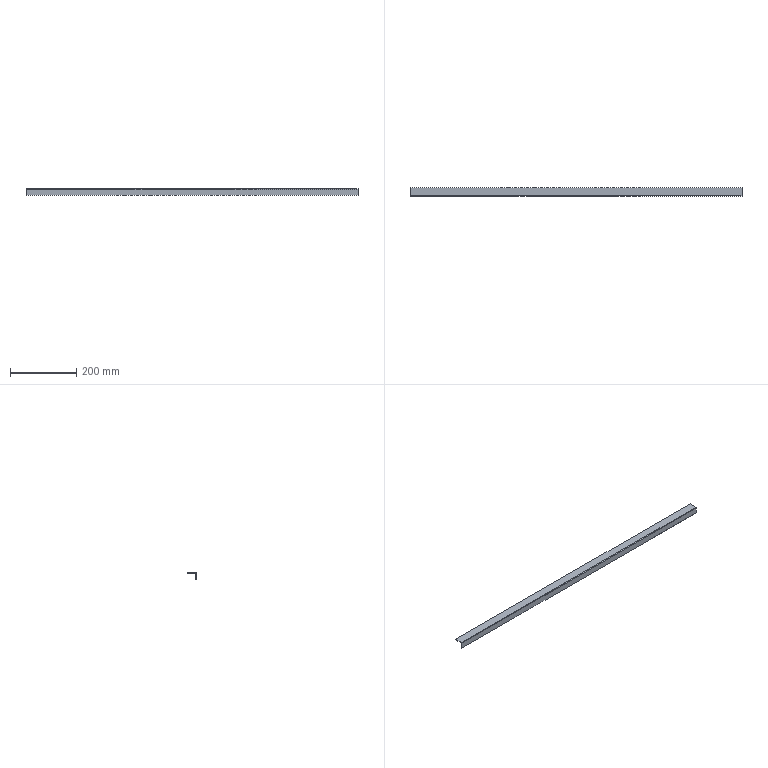Part | SolidWorks | features SplitBody 1 | 1 solid | 14 faces | box 1000 x 26.5 x 20 mm | volume 66953 mm3 | plane 12 | cylinder 2 | commonest cylinder face diameters 0.2 x1 3.2 x1
STEP:
#1=CARTESIAN_POINT('',(-500.,1.5,273.4));
#2=VERTEX_POINT('',#1);
#3=CARTESIAN_POINT('',(-500.,0.,273.4));
#4=VERTEX_POINT('',#3);
#5=CARTESIAN_POINT('',(-500.,1.5,273.4));
#6=DIRECTION('',(0.,-1.,0.));
#7=VECTOR('',#6,1000.);
#8=LINE('',#5,#7);
#9=EDGE_CURVE('',#2,#4,#8,.T.);
#10=ORIENTED_EDGE('',*,*,#9,.F.);
#11=CARTESIAN_POINT('',(-500.,1.5,255.));
#12=VERTEX_POINT('',#11);
#13=CARTESIAN_POINT('',(-500.,1.5,255.));
#14=DIRECTION('',(0.,0.,1.));
#15=VECTOR('',#14,1000.);
#16=LINE('',#13,#15);
#17=EDGE_CURVE('',#12,#2,#16,.T.);
#18=ORIENTED_EDGE('',*,*,#17,.F.);
#19=CARTESIAN_POINT('',(-500.,0.,255.));
#20=VERTEX_POINT('',#19);
#21=CARTESIAN_POINT('',(-500.,1.5,255.));
#22=DIRECTION('',(0.,-1.,0.));
#23=VECTOR('',#22,1000.);
#24=LINE('',#21,#23);
#25=EDGE_CURVE('',#12,#20,#24,.T.);
#26=ORIENTED_EDGE('',*,*,#25,.T.);
#27=CARTESIAN_POINT('',(-500.,0.,255.));
#28=DIRECTION('',(0.,0.,1.));
#29=VECTOR('',#28,1000.);
#30=LINE('',#27,#29);
#31=EDGE_CURVE('',#20,#4,#30,.T.);
#32=ORIENTED_EDGE('',*,*,#31,.T.);
#33=EDGE_LOOP('',(#10,#18,#26,#32));
#34=FACE_OUTER_BOUND('',#33,.T.);
#35=CARTESIAN_POINT('',(-500.,1.5,255.));
#36=DIRECTION('',(1.,0.,0.));
#37=DIRECTION('',(0.,0.,-1.));
#38=AXIS2_PLACEMENT_3D('',#35,#36,#37);
#39=PLANE('',#38);
#40=ADVANCED_FACE('',(#34),#39,.F.);
#41=CARTESIAN_POINT('',(500.,1.5,273.4));
#42=VERTEX_POINT('',#41);
#43=CARTESIAN_POINT('',(500.,0.,273.4));
#44=VERTEX_POINT('',#43);
#45=CARTESIAN_POINT('',(500.,1.5,273.4));
#46=DIRECTION('',(0.,-1.,0.));
#47=VECTOR('',#46,1000.);
#48=LINE('',#45,#47);
#49=EDGE_CURVE('',#42,#44,#48,.T.);
#50=ORIENTED_EDGE('',*,*,#49,.T.);
#51=CARTESIAN_POINT('',(500.,0.,255.));
#52=VERTEX_POINT('',#51);
#53=CARTESIAN_POINT('',(500.,0.,255.));
#54=DIRECTION('',(0.,0.,-1.));
#55=VECTOR('',#54,1000.);
#56=LINE('',#53,#55);
#57=EDGE_CURVE('',#44,#52,#56,.T.);
#58=ORIENTED_EDGE('',*,*,#57,.T.);
#59=CARTESIAN_POINT('',(500.,1.5,255.));
#60=VERTEX_POINT('',#59);
#61=CARTESIAN_POINT('',(500.,1.5,255.));
#62=DIRECTION('',(0.,-1.,0.));
#63=VECTOR('',#62,1000.);
#64=LINE('',#61,#63);
#65=EDGE_CURVE('',#60,#52,#64,.T.);
#66=ORIENTED_EDGE('',*,*,#65,.F.);
#67=CARTESIAN_POINT('',(500.,1.5,255.));
#68=DIRECTION('',(0.,0.,-1.));
#69=VECTOR('',#68,1000.);
#70=LINE('',#67,#69);
#71=EDGE_CURVE('',#42,#60,#70,.T.);
#72=ORIENTED_EDGE('',*,*,#71,.F.);
#73=EDGE_LOOP('',(#50,#58,#66,#72));
#74=FACE_OUTER_BOUND('',#73,.T.);
#75=CARTESIAN_POINT('',(500.,1.5,255.));
#76=DIRECTION('',(-1.,0.,0.));
#77=DIRECTION('',(0.,0.,1.));
#78=AXIS2_PLACEMENT_3D('',#75,#76,#77);
#79=PLANE('',#78);
#80=ADVANCED_FACE('',(#74),#79,.F.);
#81=ORIENTED_EDGE('',*,*,#17,.T.);
#82=CARTESIAN_POINT('',(500.,1.5,273.4));
#83=DIRECTION('',(-1.,0.,0.));
#84=VECTOR('',#83,1000.);
#85=LINE('',#82,#84);
#86=EDGE_CURVE('',#42,#2,#85,.T.);
#87=ORIENTED_EDGE('',*,*,#86,.F.);
#88=ORIENTED_EDGE('',*,*,#71,.T.);
#89=CARTESIAN_POINT('',(-500.,1.5,255.));
#90=DIRECTION('',(-1.,0.,0.));
#91=VECTOR('',#90,1000.);
#92=LINE('',#89,#91);
#93=EDGE_CURVE('',#60,#12,#92,.T.);
#94=ORIENTED_EDGE('',*,*,#93,.T.);
#95=EDGE_LOOP('',(#81,#87,#88,#94));
#96=FACE_OUTER_BOUND('',#95,.T.);
#97=CARTESIAN_POINT('',(0.,1.5,0.));
#98=DIRECTION('',(0.,1.,0.));
#99=DIRECTION('',(0.,0.,1.));
#100=AXIS2_PLACEMENT_3D('',#97,#98,#99);
#101=PLANE('',#100);
#102=ADVANCED_FACE('',(#96),#101,.T.);
#103=CARTESIAN_POINT('',(500.,0.,273.4));
#104=DIRECTION('',(-1.,0.,0.));
#105=VECTOR('',#104,1000.);
#106=LINE('',#103,#105);
#107=EDGE_CURVE('',#44,#4,#106,.T.);
#108=ORIENTED_EDGE('',*,*,#107,.T.);
#109=ORIENTED_EDGE('',*,*,#31,.F.);
#110=CARTESIAN_POINT('',(-500.,0.,255.));
#111=DIRECTION('',(-1.,0.,0.));
#112=VECTOR('',#111,1000.);
#113=LINE('',#110,#112);
#114=EDGE_CURVE('',#52,#20,#113,.T.);
#115=ORIENTED_EDGE('',*,*,#114,.F.);
#116=ORIENTED_EDGE('',*,*,#57,.F.);
#117=EDGE_LOOP('',(#108,#109,#115,#116));
#118=FACE_OUTER_BOUND('',#117,.T.);
#119=CARTESIAN_POINT('',(0.,0.,0.));
#120=DIRECTION('',(0.,1.,0.));
#121=DIRECTION('',(0.,0.,1.));
#122=AXIS2_PLACEMENT_3D('',#119,#120,#121);
#123=PLANE('',#122);
#124=ADVANCED_FACE('',(#118),#123,.F.);
#125=ORIENTED_EDGE('',*,*,#114,.T.);
#126=ORIENTED_EDGE('',*,*,#25,.F.);
#127=ORIENTED_EDGE('',*,*,#93,.F.);
#128=ORIENTED_EDGE('',*,*,#65,.T.);
#129=EDGE_LOOP('',(#125,#126,#127,#128));
#130=FACE_OUTER_BOUND('',#129,.T.);
#131=CARTESIAN_POINT('',(-500.,1.5,255.));
#132=DIRECTION('',(0.,0.,1.));
#133=DIRECTION('',(1.,0.,0.));
#134=AXIS2_PLACEMENT_3D('',#131,#132,#133);
#135=PLANE('',#134);
#136=ADVANCED_FACE('',(#130),#135,.F.);
#137=CARTESIAN_POINT('',(-500.,1.6,273.5));
#138=VERTEX_POINT('',#137);
#139=CARTESIAN_POINT('',(-500.,1.6,275.));
#140=VERTEX_POINT('',#139);
#141=CARTESIAN_POINT('',(-500.,1.6,275.));
#142=DIRECTION('',(0.,0.,1.));
#143=VECTOR('',#142,1000.);
#144=LINE('',#141,#143);
#145=EDGE_CURVE('',#138,#140,#144,.T.);
#146=ORIENTED_EDGE('',*,*,#145,.F.);
#147=CARTESIAN_POINT('',(-500.,1.6,273.4));
#148=DIRECTION('',(-1.,0.,0.));
#149=DIRECTION('',(0.,0.,-1.));
#150=AXIS2_PLACEMENT_3D('',#147,#148,#149);
#151=CIRCLE('',#150,0.1);
#152=EDGE_CURVE('',#2,#138,#151,.T.);
#153=ORIENTED_EDGE('',*,*,#152,.F.);
#154=ORIENTED_EDGE('',*,*,#9,.T.);
#155=CARTESIAN_POINT('',(-500.,1.6,273.4));
#156=DIRECTION('',(-1.,0.,0.));
#157=DIRECTION('',(0.,0.,-1.));
#158=AXIS2_PLACEMENT_3D('',#155,#156,#157);
#159=CIRCLE('',#158,1.6);
#160=EDGE_CURVE('',#4,#140,#159,.T.);
#161=ORIENTED_EDGE('',*,*,#160,.T.);
#162=EDGE_LOOP('',(#146,#153,#154,#161));
#163=FACE_OUTER_BOUND('',#162,.T.);
#164=CARTESIAN_POINT('',(-500.,1.6,273.4));
#165=DIRECTION('',(-1.,0.,0.));
#166=DIRECTION('',(0.,0.,1.));
#167=AXIS2_PLACEMENT_3D('',#164,#165,#166);
#168=PLANE('',#167);
#169=ADVANCED_FACE('',(#163),#168,.T.);
#170=CARTESIAN_POINT('',(500.,1.6,273.5));
#171=VERTEX_POINT('',#170);
#172=CARTESIAN_POINT('',(500.,1.6,273.4));
#173=DIRECTION('',(1.,0.,0.));
#174=DIRECTION('',(0.,0.,-1.));
#175=AXIS2_PLACEMENT_3D('',#172,#173,#174);
#176=CIRCLE('',#175,0.1);
#177=EDGE_CURVE('',#171,#42,#176,.T.);
#178=ORIENTED_EDGE('',*,*,#177,.F.);
#179=CARTESIAN_POINT('',(500.,1.6,275.));
#180=VERTEX_POINT('',#179);
#181=CARTESIAN_POINT('',(500.,1.6,273.5));
#182=DIRECTION('',(0.,0.,1.));
#183=VECTOR('',#182,1000.);
#184=LINE('',#181,#183);
#185=EDGE_CURVE('',#171,#180,#184,.T.);
#186=ORIENTED_EDGE('',*,*,#185,.T.);
#187=CARTESIAN_POINT('',(500.,1.6,273.4));
#188=DIRECTION('',(1.,0.,0.));
#189=DIRECTION('',(0.,0.,-1.));
#190=AXIS2_PLACEMENT_3D('',#187,#188,#189);
#191=CIRCLE('',#190,1.6);
#192=EDGE_CURVE('',#180,#44,#191,.T.);
#193=ORIENTED_EDGE('',*,*,#192,.T.);
#194=ORIENTED_EDGE('',*,*,#49,.F.);
#195=EDGE_LOOP('',(#178,#186,#193,#194));
#196=FACE_OUTER_BOUND('',#195,.T.);
#197=CARTESIAN_POINT('',(500.,1.6,273.4));
#198=DIRECTION('',(-1.,0.,0.));
#199=DIRECTION('',(0.,0.,1.));
#200=AXIS2_PLACEMENT_3D('',#197,#198,#199);
#201=PLANE('',#200);
#202=ADVANCED_FACE('',(#196),#201,.F.);
#203=ORIENTED_EDGE('',*,*,#107,.F.);
#204=ORIENTED_EDGE('',*,*,#192,.F.);
#205=CARTESIAN_POINT('',(-500.,1.6,275.));
#206=DIRECTION('',(-1.,0.,0.));
#207=VECTOR('',#206,1000.);
#208=LINE('',#205,#207);
#209=EDGE_CURVE('',#180,#140,#208,.T.);
#210=ORIENTED_EDGE('',*,*,#209,.T.);
#211=ORIENTED_EDGE('',*,*,#160,.F.);
#212=EDGE_LOOP('',(#203,#204,#210,#211));
#213=FACE_OUTER_BOUND('',#212,.T.);
#214=CARTESIAN_POINT('',(500.,1.6,273.4));
#215=DIRECTION('',(1.,0.,0.));
#216=DIRECTION('',(0.,0.,1.));
#217=AXIS2_PLACEMENT_3D('',#214,#215,#216);
#218=CYLINDRICAL_SURFACE('',#217,1.6);
#219=ADVANCED_FACE('',(#213),#218,.T.);
#220=ORIENTED_EDGE('',*,*,#86,.T.);
#221=ORIENTED_EDGE('',*,*,#152,.T.);
#222=CARTESIAN_POINT('',(-500.,1.6,273.5));
#223=DIRECTION('',(1.,0.,0.));
#224=VECTOR('',#223,1000.);
#225=LINE('',#222,#224);
#226=EDGE_CURVE('',#138,#171,#225,.T.);
#227=ORIENTED_EDGE('',*,*,#226,.T.);
#228=ORIENTED_EDGE('',*,*,#177,.T.);
#229=EDGE_LOOP('',(#220,#221,#227,#228));
#230=FACE_OUTER_BOUND('',#229,.T.);
#231=CARTESIAN_POINT('',(500.,1.6,273.4));
#232=DIRECTION('',(1.,0.,0.));
#233=DIRECTION('',(0.,0.,1.));
#234=AXIS2_PLACEMENT_3D('',#231,#232,#233);
#235=CYLINDRICAL_SURFACE('',#234,0.1);
#236=ADVANCED_FACE('',(#230),#235,.F.);
#237=ORIENTED_EDGE('',*,*,#145,.T.);
#238=CARTESIAN_POINT('',(-500.,26.5,275.));
#239=VERTEX_POINT('',#238);
#240=CARTESIAN_POINT('',(-500.,0.,275.));
#241=DIRECTION('',(0.,-1.,0.));
#242=VECTOR('',#241,1000.);
#243=LINE('',#240,#242);
#244=EDGE_CURVE('',#239,#140,#243,.T.);
#245=ORIENTED_EDGE('',*,*,#244,.F.);
#246=CARTESIAN_POINT('',(-500.,26.5,273.5));
#247=VERTEX_POINT('',#246);
#248=CARTESIAN_POINT('',(-500.,26.5,275.));
#249=DIRECTION('',(0.,0.,-1.));
#250=VECTOR('',#249,1000.);
#251=LINE('',#248,#250);
#252=EDGE_CURVE('',#239,#247,#251,.T.);
#253=ORIENTED_EDGE('',*,*,#252,.T.);
#254=CARTESIAN_POINT('',(-500.,1.5,273.5));
#255=DIRECTION('',(0.,-1.,0.));
#256=VECTOR('',#255,1000.);
#257=LINE('',#254,#256);
#258=EDGE_CURVE('',#247,#138,#257,.T.);
#259=ORIENTED_EDGE('',*,*,#258,.T.);
#260=EDGE_LOOP('',(#237,#245,#253,#259));
#261=FACE_OUTER_BOUND('',#260,.T.);
#262=CARTESIAN_POINT('',(-500.,1.5,275.));
#263=DIRECTION('',(1.,0.,0.));
#264=DIRECTION('',(0.,1.,0.));
#265=AXIS2_PLACEMENT_3D('',#262,#263,#264);
#266=PLANE('',#265);
#267=ADVANCED_FACE('',(#261),#266,.F.);
#268=ORIENTED_EDGE('',*,*,#185,.F.);
#269=CARTESIAN_POINT('',(500.,26.5,273.5));
#270=VERTEX_POINT('',#269);
#271=CARTESIAN_POINT('',(500.,26.5,273.5));
#272=DIRECTION('',(0.,1.,0.));
#273=VECTOR('',#272,1000.);
#274=LINE('',#271,#273);
#275=EDGE_CURVE('',#171,#270,#274,.T.);
#276=ORIENTED_EDGE('',*,*,#275,.T.);
#277=CARTESIAN_POINT('',(500.,26.5,275.));
#278=VERTEX_POINT('',#277);
#279=CARTESIAN_POINT('',(500.,26.5,275.));
#280=DIRECTION('',(0.,0.,-1.));
#281=VECTOR('',#280,1000.);
#282=LINE('',#279,#281);
#283=EDGE_CURVE('',#278,#270,#282,.T.);
#284=ORIENTED_EDGE('',*,*,#283,.F.);
#285=CARTESIAN_POINT('',(500.,0.,275.));
#286=DIRECTION('',(0.,1.,0.));
#287=VECTOR('',#286,1000.);
#288=LINE('',#285,#287);
#289=EDGE_CURVE('',#180,#278,#288,.T.);
#290=ORIENTED_EDGE('',*,*,#289,.F.);
#291=EDGE_LOOP('',(#268,#276,#284,#290));
#292=FACE_OUTER_BOUND('',#291,.T.);
#293=CARTESIAN_POINT('',(500.,26.5,275.));
#294=DIRECTION('',(-1.,0.,0.));
#295=DIRECTION('',(0.,-1.,0.));
#296=AXIS2_PLACEMENT_3D('',#293,#294,#295);
#297=PLANE('',#296);
#298=ADVANCED_FACE('',(#292),#297,.F.);
#299=ORIENTED_EDGE('',*,*,#209,.F.);
#300=ORIENTED_EDGE('',*,*,#289,.T.);
#301=CARTESIAN_POINT('',(0.,26.5,275.));
#302=DIRECTION('',(-1.,0.,0.));
#303=VECTOR('',#302,1000.);
#304=LINE('',#301,#303);
#305=EDGE_CURVE('',#278,#239,#304,.T.);
#306=ORIENTED_EDGE('',*,*,#305,.T.);
#307=ORIENTED_EDGE('',*,*,#244,.T.);
#308=EDGE_LOOP('',(#299,#300,#306,#307));
#309=FACE_OUTER_BOUND('',#308,.T.);
#310=CARTESIAN_POINT('',(0.,0.,275.));
#311=DIRECTION('',(0.,0.,-1.));
#312=DIRECTION('',(-1.,0.,0.));
#313=AXIS2_PLACEMENT_3D('',#310,#311,#312);
#314=PLANE('',#313);
#315=ADVANCED_FACE('',(#309),#314,.F.);
#316=ORIENTED_EDGE('',*,*,#275,.F.);
#317=ORIENTED_EDGE('',*,*,#226,.F.);
#318=ORIENTED_EDGE('',*,*,#258,.F.);
#319=CARTESIAN_POINT('',(-500.,26.5,273.5));
#320=DIRECTION('',(-1.,0.,0.));
#321=VECTOR('',#320,1000.);
#322=LINE('',#319,#321);
#323=EDGE_CURVE('',#270,#247,#322,.T.);
#324=ORIENTED_EDGE('',*,*,#323,.F.);
#325=EDGE_LOOP('',(#316,#317,#318,#324));
#326=FACE_OUTER_BOUND('',#325,.T.);
#327=CARTESIAN_POINT('',(0.,0.,273.5));
#328=DIRECTION('',(0.,0.,-1.));
#329=DIRECTION('',(-1.,0.,0.));
#330=AXIS2_PLACEMENT_3D('',#327,#328,#329);
#331=PLANE('',#330);
#332=ADVANCED_FACE('',(#326),#331,.T.);
#333=ORIENTED_EDGE('',*,*,#323,.T.);
#334=ORIENTED_EDGE('',*,*,#252,.F.);
#335=ORIENTED_EDGE('',*,*,#305,.F.);
#336=ORIENTED_EDGE('',*,*,#283,.T.);
#337=EDGE_LOOP('',(#333,#334,#335,#336));
#338=FACE_OUTER_BOUND('',#337,.T.);
#339=CARTESIAN_POINT('',(-500.,26.5,275.));
#340=DIRECTION('',(0.,-1.,0.));
#341=DIRECTION('',(0.,0.,-1.));
#342=AXIS2_PLACEMENT_3D('',#339,#340,#341);
#343=PLANE('',#342);
#344=ADVANCED_FACE('',(#338),#343,.F.);
#345=CLOSED_SHELL('',(#40,#80,#102,#124,#136,#169,#202,#219,#236,#267,#298,#315,#332,#344));
#346=MANIFOLD_SOLID_BREP('',#345);
#347=CARTESIAN_POINT('',(0.,0.,0.));
#348=DIRECTION('',(0.,0.,1.));
#349=DIRECTION('',(1.,0.,0.));
#350=AXIS2_PLACEMENT_3D('',#347,#348,#349);
#351=(LENGTH_UNIT()NAMED_UNIT(*)SI_UNIT(.MILLI.,.METRE.));
#352=UNCERTAINTY_MEASURE_WITH_UNIT(LENGTH_MEASURE(0.00001),#351,'','');
#353=(NAMED_UNIT(*)PLANE_ANGLE_UNIT()SI_UNIT($,.RADIAN.));
#354=(NAMED_UNIT(*)SI_UNIT($,.STERADIAN.)SOLID_ANGLE_UNIT());
#355=(GEOMETRIC_REPRESENTATION_CONTEXT(3)GLOBAL_UNCERTAINTY_ASSIGNED_CONTEXT((#352))GLOBAL_UNIT_ASSIGNED_CONTEXT((#351,#353,#354))REPRESENTATION_CONTEXT('',''));
#356=ADVANCED_BREP_SHAPE_REPRESENTATION('',(#346,#350),#355);